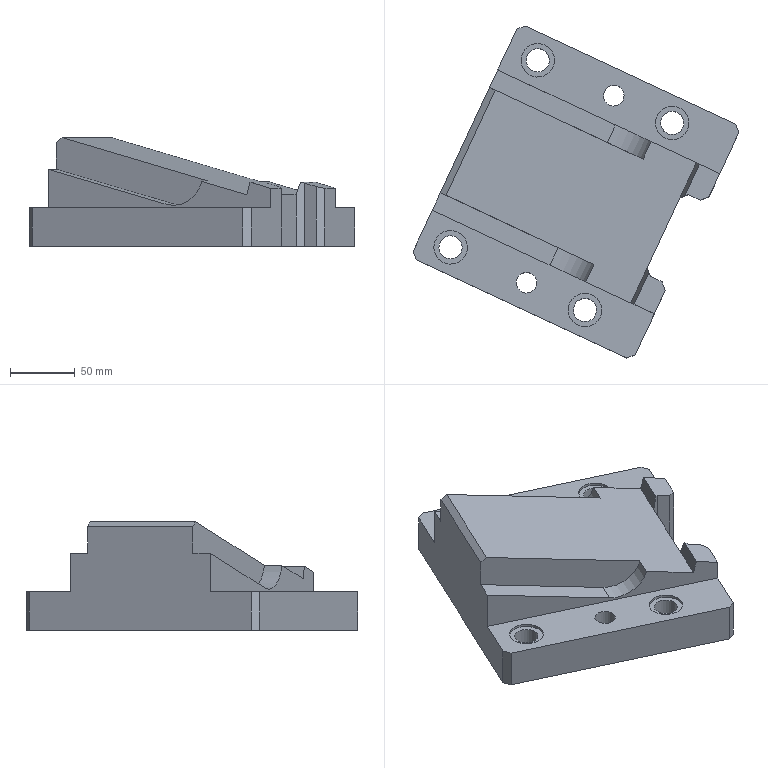Part | NX | features solid 2 | 1 solid | 68 faces | box 252.496 x 257.333 x 84.257 mm | volume 1585768 mm3 | plane 56 | cylinder 12 | commonest cylinder face diameters 18 x4 26 x4 16 x2 50 x2